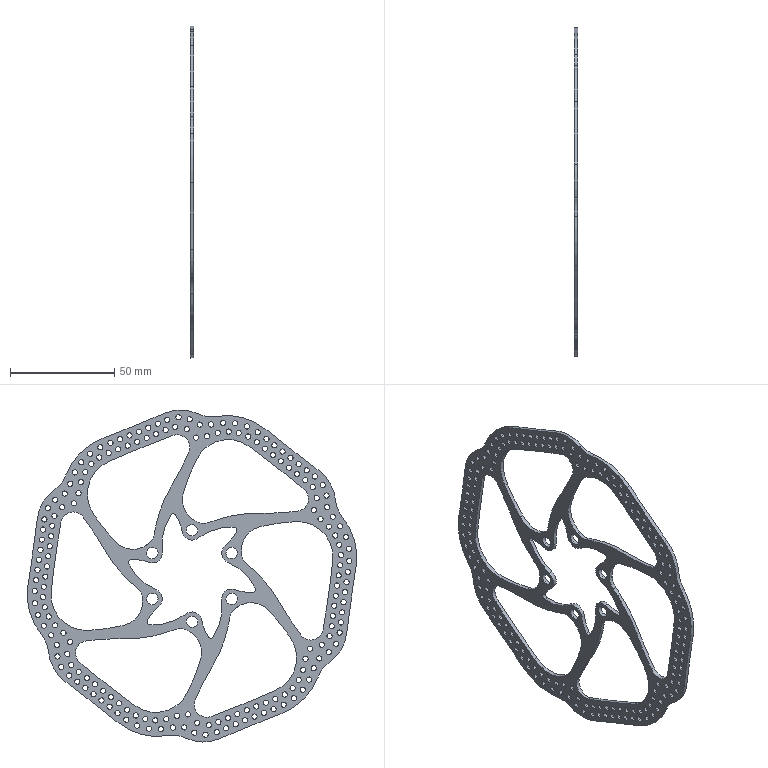Part | STEP file | BREP_51 | 1 solid | 485 faces | box 1.8 x 158.335 x 159.5 mm | volume 12555 mm3 | cylinder 475 | plane 8 | other 2 | commonest cylinder face diameters 2.5 x360 5.5 x12 2.8 x4 12 x4 9.5 x3 23.002 x3